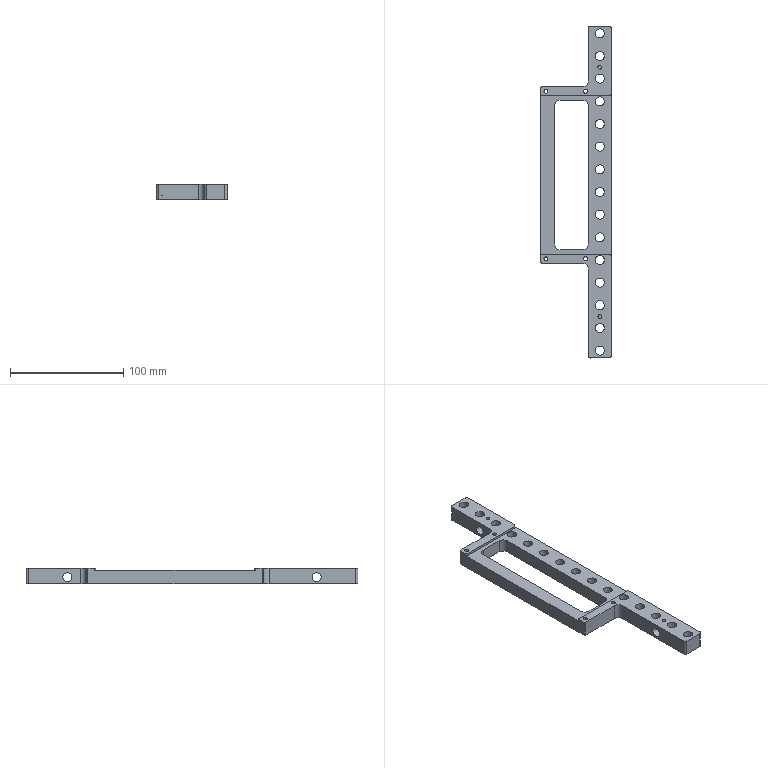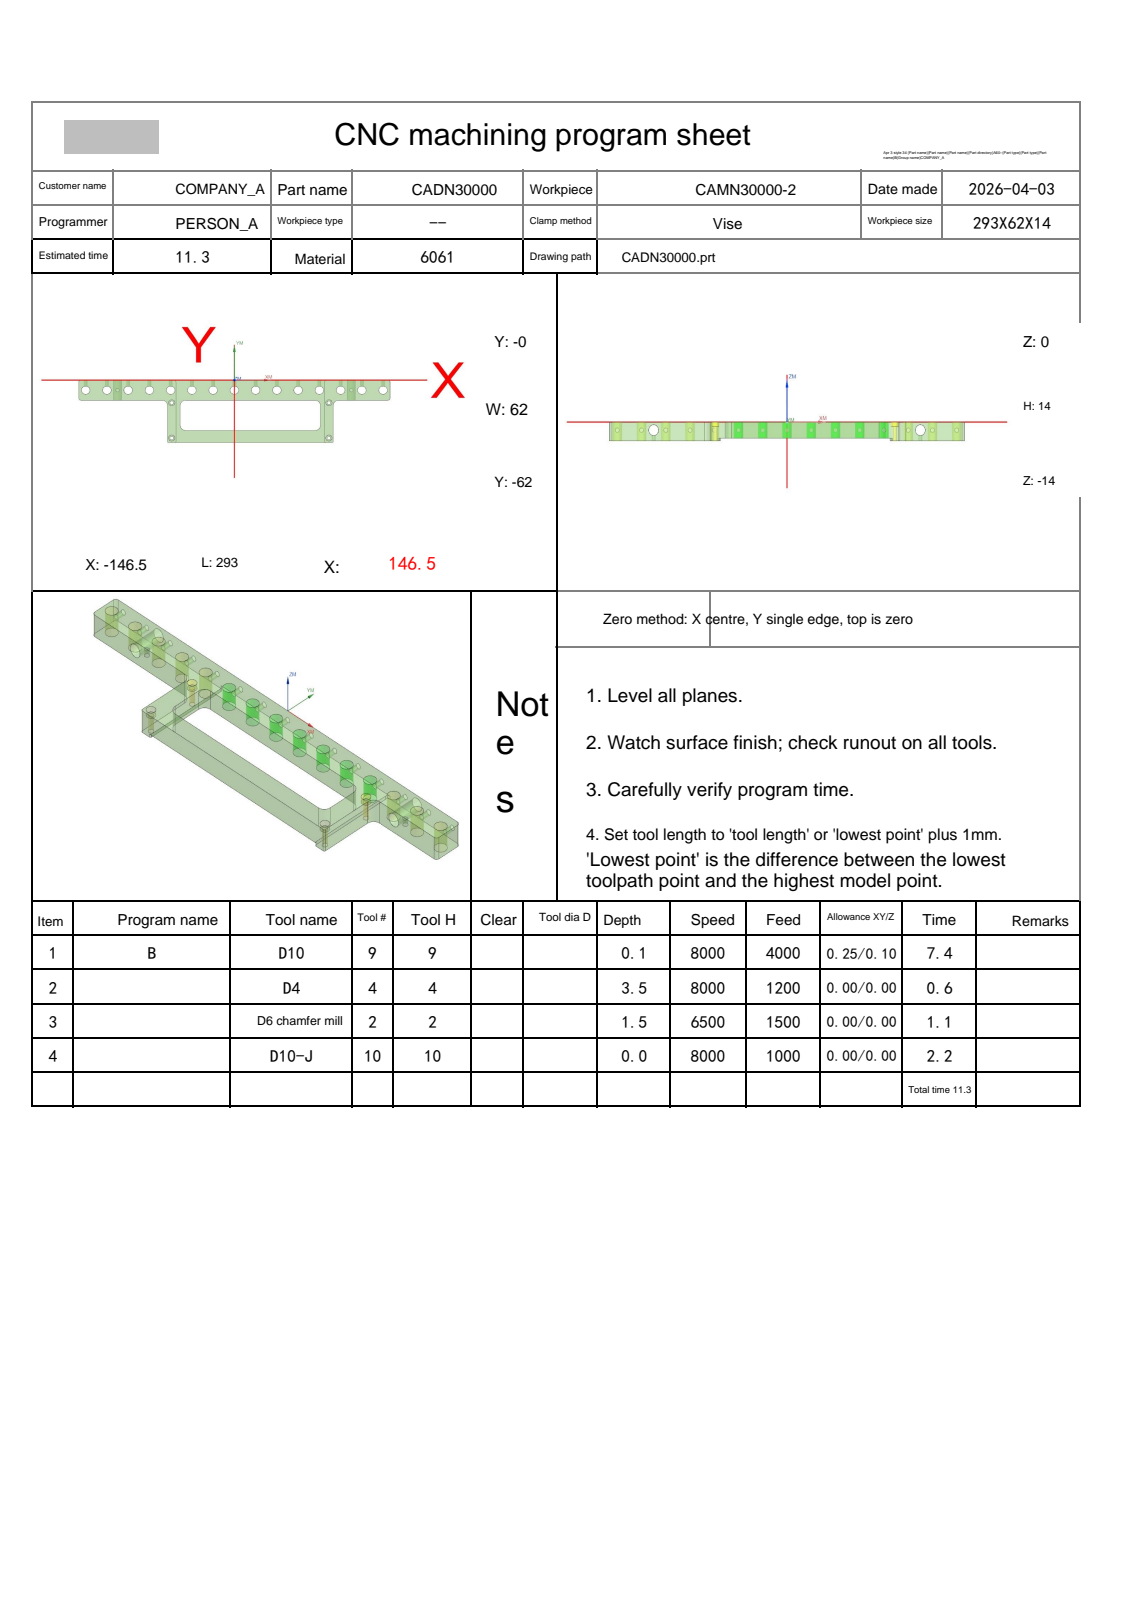NC program | NX | posted by the shop | part box 62 x 293 x 14 mm
Lines 1 to 1541 of 1949, first 1264 of 1539 lines:
%
O0001
(Machine time: 11.99 MIN)
(===Total Tool:4===)
(T9=D10     D=10.  R=0.   D-  H09 Z=0.1   )
(T4=D4      D=4.   R=0.   D-  H04 Z=-3.5  )
(T2=D6 chamfer mill   D=6.   R=0.   D-  H02 Z=-1.5  )
(T10=D10-J  D=10.  R=0.   D-  H10 Z=-0.   )
G80 G90 G17 G49 G40
G91 G28 Z0
M01
N1 T09 M06
(D10  D=10. R=0. H=09 ce=0.25 di=0.10)
G00 G90 G54 X88.84 Y12.6 M03 S8000
G43 H09 Z20.
M08
Z2.1
G01 X88.857 Y12.502 Z1.476 F4000.
X88.874 Y12.403 Z1.228
X88.891 Y12.305 Z1.046
X88.908 Y12.206 Z.9
X88.925 Y12.108 Z.777
X88.943 Y12.009 Z.672
X88.96 Y11.911 Z.58
X88.977 Y11.812 Z.5
X88.994 Y11.714 Z.43
X89.011 Y11.615 Z.368
X89.028 Y11.516 Z.314
X89.045 Y11.418 Z.267
X89.062 Y11.319 Z.227
X89.079 Y11.221 Z.192
X89.096 Y11.122 Z.164
X89.113 Y11.024 Z.14
X89.13 Y10.925 Z.123
X89.147 Y10.827 Z.11
X89.164 Y10.728 Z.103
X89.181 Y10.63 Z.1
X89.568 Y8.389
G03 X89.885 Y8.003 I.502 J.09
X93.672 Y7.43 I3.807 J12.364
X102.367 Y7.294 I8.695 J277.549
X104.221 Y7.3 I0.0 J277.686
G01 X147.34 Y7.279
G02 X153.274 Y3.249 I-.2 J-6.678
X154.598 Y-2.599 I-14.948 J-6.46
X154.816 Y-11.507 I-182.121 J-8.909
X154.799 Y-14.005 I-182.338 J0.0
G01 X154.782 Y-61.787
G02 X150.627 Y-67.842 I-6.717 J.156
X144.706 Y-69.114 I-6.461 J15.657
X136.65 Y-69.305 I-8.056 J169.876
X135.049 Y-69.297 I0.0 J170.067
G01 X-147.307 Y-69.281
G02 X-153.303 Y-65.187 I.18 J6.701
X-154.592 Y-59.479 I14.994 J6.386
X-154.808 Y-51.337 I153.279 J8.142
X-154.798 Y-49.543 I153.495 J0.0
G01 X-154.781 Y-.193
G02 X-150.823 Y5.737 I6.655 J-.155
X-145.06 Y7.085 I6.436 J-14.522
X-136.504 Y7.313 I8.556 J-160.42
X-134.285 Y7.298 I0.0 J-160.648
G01 X87.395 Y7.279
G03 X96.14 Y6.68 I14.491 J147.608
X105.341 Y6.601 I9.81 J603.736
G01 X145.58 Y6.575
G02 X152.002 Y2.432 I-.439 J-7.729
X153.748 Y-3.652 I-14.055 J-7.328
X154.101 Y-11.947 I-97.334 J-8.296
X154.092 Y-13.301 I-97.687 J0.0
G01 X154.082 Y-59.92
G02 X149.837 Y-66.561 I-7.749 J.276
X143.738 Y-68.262 I-7.302 J14.397
X135.453 Y-68.601 I-8.285 J101.008
X134.088 Y-68.592 I0.0 J101.348
G01 X-145.58 Y-68.575
G02 X-152.029 Y-64.382 I.448 J7.745
X-153.755 Y-58.288 I14.212 J7.317
X-154.11 Y-49.527 I108.129 J8.761
X-154.095 Y-47.728 I108.483 J0.0
G01 X-154.075 Y-1.921
G02 X-149.934 Y4.499 I7.732 J-.442
X-143.711 Y6.263 I7.389 J-14.205
X-135.007 Y6.609 I8.704 J-109.461
X-133.221 Y6.594 I0.0 J-109.807
G01 X85.659 Y6.584
G02 X94.023 Y6.08 I-43.845 J-798.073
G03 X105.145 Y5.898 I11.123 J339.757
X106.531 Y5.901 I0.0 J339.939
G01 X143.761 Y5.877
G02 X151.325 Y.864 I-.379 J-8.787
X153.058 Y-5.735 I-16.655 J-7.9
X153.409 Y-15.038 I-123.06 J-9.303
X153.395 Y-16.926 I-123.411 J0.0
G01 X153.375 Y-58.285
G02 X148.444 Y-65.787 I-8.757 J.384
X141.717 Y-67.564 I-7.966 J16.537
X132.386 Y-67.909 I-9.331 J125.76
X130.456 Y-67.895 I0.0 J126.105
G01 X-143.723 Y-67.877
G02 X-151.337 Y-62.841 I.347 J8.797
X-153.067 Y-56.172 I16.812 J7.921
X-153.409 Y-46.885 I126.17 J9.288
X-153.395 Y-44.981 I126.512 J0.0
G01 X-153.377 Y-3.761
G02 X-148.442 Y3.784 I8.769 J-.349
X-141.847 Y5.549 I7.91 J-16.351
X-133.209 Y5.897 I8.638 J-107.04
X-131.987 Y5.89 I0.0 J-107.388
G01 X84.723 Y5.876
G02 X94.905 Y5.361 I-44.85 J-988.753
G03 X107.105 Y5.198 I12.2 J456.693
X108.841 Y5.202 I0.0 J456.856
G01 X142.01 Y5.179
G02 X150.616 Y-.477 I-.151 J-9.604
X152.35 Y-7.374 I-18.435 J-8.3
X152.71 Y-17.163 I-132.671 J-9.789
X152.695 Y-19.195 I-133.032 J0.0
G01 X152.678 Y-56.495
G02 X147.046 Y-65.107 I-9.589 J.123
X140.091 Y-66.854 I-8.325 J18.431
X130.3 Y-67.21 I-9.791 J134.473
X128.27 Y-67.194 I0.0 J134.829
G01 X-141.99 Y-67.177
G02 X-150.618 Y-61.517 I.129 J9.603
X-152.37 Y-54.413 I18.732 J8.387
X-152.702 Y-45.095 I130.593 J9.318
X-152.693 Y-43.501 I130.925 J0.0
G01 X-152.677 Y-5.501
G02 X-147.023 Y3.116 I9.604 J-.138
X-140.126 Y4.849 I8.3 J-18.445
X-130.723 Y5.203 I9.403 J-124.716
X-129.075 Y5.192 I0.0 J-125.07
G01 X83.715 Y5.175
G02 X94.918 Y4.674 I-31.295 J-824.645
G03 X108.198 Y4.496 I13.28 J497.487
X110.451 Y4.502 I0.0 J497.664
G01 X140.4 Y4.479
X140.468 Y4.48
G02 X149.953 Y-1.808 I0.0 J-10.298
X151.663 Y-9.069 I-20.482 J-8.658
X152.004 Y-18.858 I-140.517 J-9.788
X151.993 Y-20.611 I-140.858 J0.0
G01 X151.98 Y-54.831
X151.981 Y-54.97
G02 X148.938 Y-62.275 I-10.291 J0.0
X142.504 Y-65.531 I-9.145 J10.086
X133.954 Y-66.411 I-8.704 J42.604
X122.796 Y-66.502 I-11.158 J686.931
X120.655 Y-66.498 I0.0 J687.022
G01 X-140.295 Y-66.481
X-140.451 Y-66.482
G02 X-147.553 Y-63.657 I0.0 J10.341
X-151.023 Y-57.031 I9.674 J9.288
X-151.912 Y-48.412 I42.61 J8.75
X-152.002 Y-37.319 I686.42 J11.093
X-151.998 Y-35.183 I686.51 J0.0
G01 X-151.975 Y-7.053
Y-7.023
G02 X-145.736 Y2.433 I10.284 J0.0
X-138.343 Y4.171 I8.722 J-20.502
X-128.525 Y4.504 I9.818 J-144.463
X-126.731 Y4.493 I0.0 J-144.796
G01 X82.559 Y4.479
G02 X95.738 Y3.957 I-29.69 J-915.635
G03 X109.111 Y3.801 I13.373 J573.724
X110.241 Y3.802 I0.0 J573.88
G01 X138.93 Y3.779
X139.056
G02 X145.641 Y1.684 I0.0 J-11.398
X149.894 Y-4.682 I-7.718 J-9.76
X151.13 Y-12.967 I-31.784 J-8.976
X151.314 Y-24.728 I-376.482 J-11.761
X151.298 Y-28.155 I-376.666 J0.0
G01 X151.279 Y-53.345
X151.28 Y-53.52
G02 X149.36 Y-59.899 I-11.556 J0.0
X142.994 Y-64.339 I-9.814 J7.288
X134.787 Y-65.617 I-8.967 J30.583
X122.844 Y-65.816 I-11.944 J359.429
X119.25 Y-65.798 I0.0 J359.627
G01 X-138.83 Y-65.779
X-139.013 Y-65.78
G02 X-145.447 Y-63.823 I0.0 J11.554
X-149.891 Y-57.325 I7.423 J9.846
X-151.13 Y-49.04 I31.759 J8.982
X-151.314 Y-37.2 I380.01 J11.84
X-151.298 Y-33.712 I380.194 J0.0
G01 X-151.277 Y-8.592
X-151.278 Y-8.446
G02 X-149.201 Y-1.884 I11.406 J0.0
X-142.754 Y2.414 I9.788 J-7.698
X-134.745 Y3.619 I8.836 J-31.512
X-122.8 Y3.816 I11.946 J-362.968
X-119.208 Y3.798 I0.0 J-363.165
G01 X81.682 Y3.78
G02 X95.597 Y3.269 I-21.781 J-783.97
G03 X110.152 Y3.097 I14.555 J615.329
X112.55 Y3.102 I0.0 J615.501
G01 X137.53 Y3.079
X137.685
G02 X143.897 Y1.449 I0.0 J-12.646
X148.895 Y-4.964 I-6.518 J-10.234
X150.361 Y-13.135 I-27.913 J-9.224
X150.606 Y-23.713 I-228.264 J-10.577
X150.596 Y-25.871 I-228.509 J0.0
G01 X150.577 Y-51.971
X150.579 Y-52.167
G02 X148.98 Y-58.347 I-12.741 J0.0
X142.64 Y-63.357 I-10.219 J6.415
X134.474 Y-64.854 I-9.244 J27.407
X123.793 Y-65.107 I-10.681 J225.167
X121.528 Y-65.095 I0.0 J225.42
G01 X-137.462 Y-65.077
G02 X-137.662 Y-65.078 I-.2 J12.731
X-143.906 Y-63.442 I0.0 J12.733
X-148.872 Y-57.094 I6.52 J10.217
X-150.352 Y-48.996 I27.485 J9.206
X-150.607 Y-38.319 I223.444 J10.677
X-150.595 Y-36.05 I223.699 J0.0
G01 X-150.572 Y-9.88
X-150.573 Y-9.75
G02 X-148.751 Y-3.29 I12.364 J0.0
X-142.272 Y1.488 I10.176 J-7.017
X-134.29 Y2.865 I9.093 J-28.888
X-123.711 Y3.105 I10.579 J-233.001
X-121.554 Y3.095 I0.0 J-233.241
G01 X81.506 Y3.072
G02 X96.008 Y2.564 I-25.441 J-933.963
G03 X110.8 Y2.4 I14.791 J665.06
X112.621 Y2.402 I0.0 J665.225
G01 X136.13 Y2.38
G02 X136.35 Y2.382 I.22 J-13.999
X142.43 Y.993 I0.0 J-14.001
X148.029 Y-5.615 I-5.888 J-10.665
X149.614 Y-13.762 I-26.727 J-9.429
X149.914 Y-25.328 I-223.098 J-11.567
X149.896 Y-28.176 I-223.398 J0.0
G01 X149.87 Y-50.846
X149.871 Y-50.979
G02 X148.288 Y-57.303 I-13.428 J0.0
X141.67 Y-62.611 I-10.58 J6.412
X133.648 Y-64.121 I-9.33 J27.506
X122.041 Y-64.414 I-11.607 J230.015
X119.163 Y-64.396 I0.0 J230.308
G01 X-136.117 Y-64.376
G02 X-136.342 Y-64.378 I-.226 J14.074
X-142.355 Y-63.029 I0.0 J14.076
X-147.964 Y-56.545 I5.746 J10.639
X-149.606 Y-48.341 I26.119 J9.494
X-149.902 Y-37.833 I186.436 J10.507
X-149.893 Y-35.956 I186.732 J0.0
G01 X-149.875 Y-11.327
G02 X-149.876 Y-11.119 I13.86 J.208
X-148.438 Y-4.97 I13.861 J0.0
X-141.87 Y.533 I10.622 J-6.005
X-133.931 Y2.099 I9.336 J-26.426
X-122.586 Y2.412 I11.345 J-205.627
X-119.937 Y2.395 I0.0 J-205.939
G01 X80.743 Y2.373
G02 X96.006 Y1.87 I-21.929 J-897.113
G03 X111.368 Y1.7 I15.363 J692.97
X113.251 Y1.703 I0.0 J693.14
G01 X134.94 Y1.677
G02 X135.156 Y1.679 I.215 J-14.903
X141.327 Y.341 I0.0 J-14.904
X147.13 Y-6.162 I-5.666 J-10.896
X148.853 Y-14.207 I-25.216 J-9.608
X149.194 Y-24.497 I-154.696 J-10.291
X149.188 Y-25.889 I-155.038 J0.0
G01 X149.176 Y-49.328
G02 X149.178 Y-49.599 I-15.233 J-.271
X147.919 Y-55.664 I-15.236 J0.0
X141.254 Y-61.665 I-10.984 J5.499
X133.342 Y-63.348 I-9.53 J25.353
X122.945 Y-63.696 I-10.396 J155.45
X121.45 Y-63.688 I0.0 J155.798
G01 X-134.74 Y-63.678
G02 X-135.041 Y-63.681 I-.301 J15.542
X-141.024 Y-62.483 I0.0 J15.545
X-147.102 Y-55.9 I5.294 J10.986
X-148.846 Y-47.859 I24.933 J9.619
X-149.197 Y-37.382 I156.383 J10.477
X-149.189 Y-35.827 I156.734 J0.0
G01 X-149.174 Y-12.597
G02 X-149.176 Y-12.375 I15.13 J.223
X-147.916 Y-6.33 I15.132 J0.0
X-141.331 Y-.369 I10.951 J-5.479
X-133.076 Y1.37 I9.701 J-25.588
X-121.622 Y1.71 I11.454 J-192.661
X-119.083 Y1.694 I0.0 J-193.001
G01 X79.847 Y1.676
G02 X95.726 Y1.183 I-17.854 J-830.973
G03 X111.743 Y1. I16.017 J699.437
X113.811 Y1.003 I0.0 J699.62
G01 X133.751 Y.976
G02 X133.967 Y.978 I.217 J-15.98
X140.163 Y-.272 I0.0 J-15.981
X146.322 Y-6.909 I-5.414 J-11.201
X148.114 Y-14.939 I-24.864 J-9.764
X148.498 Y-25.765 I-152.549 J-10.826
X148.489 Y-27.459 I-152.932 J0.0
G01 X148.477 Y-48.029
G02 X148.48 Y-48.32 I-16.947 J-.291
X147.426 Y-54.203 I-16.95 J0.0
X140.619 Y-60.81 I-11.344 J4.878
X132.453 Y-62.624 I-9.826 J24.94
X121.138 Y-63.005 I-11.314 J167.762
X118.952 Y-62.991 I0.0 J168.143
G01 X-133.528 Y-62.977
G02 X-133.84 Y-62.98 I-.311 J16.739
X-139.832 Y-61.871 I0.0 J16.742
X-146.328 Y-55.072 I5.033 J11.312
X-148.14 Y-46.762 I25.364 J9.884
X-148.493 Y-36.299 I154.908 J10.464
X-148.488 Y-34.941 I155.261 J0.0
G01 X-148.469 Y-13.671
X-148.47 Y-13.481
G02 X-147.192 Y-7.263 I15.756 J0.0
X-140.432 Y-1.113 I11.22 J-5.541
X-132.25 Y.642 I9.799 J-25.742
X-121.093 Y1.003 I11.157 J-171.958
X-119.028 Y.991 I0.0 J-172.32
G01 X79.762 Y.971
G02 X96.624 Y.464 I-21.139 J-983.732
G03 X112.277 Y.3 I15.653 J748.037
X114.581 Y.303 I0.0 J748.201
G01 X132.421 Y.28
G02 X132.72 Y.283 I.299 J-17.568
X138.868 Y-.828 I0.0 J-17.571
X145.525 Y-7.656 I-4.993 J-11.526
X147.398 Y-15.88 I-24.884 J-9.993
X147.795 Y-26.763 I-148.941 J-10.883
X147.787 Y-28.33 I-149.338 J0.0
G01 X147.776 Y-46.87
G02 X147.779 Y-47.187 I-17.896 J-.317
X146.742 Y-53.19 I-17.898 J0.0
X139.839 Y-60.026 I-11.586 J4.795
X131.749 Y-61.886 I-9.936 J24.704
X120.994 Y-62.292 I-10.755 J142.146
X119.579 Y-62.285 I0.0 J142.553
G01 X-132.411 Y-62.275
G02 X-132.712 Y-62.277 I-.302 J17.679
X-138.793 Y-61.199 I0.0 J17.682
X-145.577 Y-54.22 I4.939 J11.588
X-147.423 Y-45.841 I25.625 J10.039
X-147.802 Y-34.57 I167.216 J11.271
X-147.79 Y-32.55 I167.595 J0.0
X-147.818 Y-25.468 I917.727 J7.082
X-147.749 Y-14.29 I917.754 J0.0
X-146.216 Y-7.665 I15.196 J-.027
X-139.246 Y-1.729 I11.361 J-6.281
X-130.692 Y-.023 I10.03 J-27.99
X-119.024 Y.307 I11.668 J-205.842
X-116.559 Y.293 I0.0 J-206.173
G01 X78.801 Y.275
G02 X96.138 Y-.22 I-16.782 J-892.922
G03 X112.269 Y-.397 I16.131 J732.322
X113.671 Y-.396 I0.0 J732.5
G02 X120.248 Y-.373 I6.577 J-953.697
X132.14 Y-.447 I0.0 J-953.72
X138.848 Y-1.95 I-.036 J-15.888
X144.958 Y-8.922 I-6.153 J-11.555
X146.724 Y-17.245 I-26.973 J-10.07
X147.102 Y-28.693 I-172.99 J-11.448
X147.09 Y-30.746 I-173.368 J0.0
X147.115 Y-36.628 I-678.98 J-5.881
X147.039 Y-46.836 I-679.006 J0.0
X145.425 Y-53.584 I-15.389 J.113
X138.313 Y-59.562 I-11.546 J6.516
X129.971 Y-61.247 I-10.024 J28.129
X118.505 Y-61.602 I-11.466 J185.038
X116.399 Y-61.59 I0.0 J185.393
G01 X-131.041 Y-61.579
G02 X-131.448 Y-61.583 I-.406 J19.659
X-137.519 Y-60.622 I0.0 J19.664
X-144.667 Y-53.748 I4.483 J11.815
X-146.656 Y-45.472 I24.145 J10.179
X-147.092 Y-34.477 I138.445 J10.995
X-147.084 Y-33.024 I138.881 J0.0
X-147.119 Y-25.987 I713.915 J7.037
X-147.036 Y-15.115 I713.95 J0.0
X-145.332 Y-8.25 I15.214 J-.132
X-138.254 Y-2.416 I11.493 J-6.734
X-129.699 Y-.731 I10.113 J-28.783
X-117.962 Y-.394 I11.737 J-204.191
X-115.566 Y-.408 I0.0 J-204.528
G01 X78.744 Y-.43
G02 X96.691 Y-.93 I-18.209 J-976.343
G03 X112.38 Y-1.097 I15.688 J736.431
X113.952 Y-1.096 I0.0 J736.598
G02 X119.766 Y-1.076 I5.815 J-886.428
X131.09 Y-1.149 I0.0 J-886.447
X137.879 Y-2.621 I-.036 J-16.56
X144.238 Y-9.806 I-6.085 J-11.791
X146.033 Y-18.415 I-27.816 J-10.293
X146.399 Y-29.803 I-177.212 J-11.388
X146.389 Y-31.707 I-177.578 J0.0
X146.416 Y-36.797 I-477.543 J-5.09
X146.328 Y-45.976 I-477.571 J0.0
X144.631 Y-52.851 I-15.592 J.2
X137.496 Y-58.815 I-11.676 J6.718
X128.881 Y-60.55 I-10.255 J28.671
X117.36 Y-60.901 I-11.521 J188.871
X115.308 Y-60.889 I0.0 J189.222
G01 X-130.102 Y-60.874
G02 X-130.451 Y-60.877 I-.349 J20.105
X-136.649 Y-59.898 I0.0 J20.108
X-144.034 Y-52.674 I4.584 J12.072
X-145.986 Y-44.108 I25.711 J10.367
X-146.393 Y-32.944 I152.908 J11.164
X-146.385 Y-31.378 I153.315 J0.0
X-146.411 Y-25.725 I615.598 J5.653
X-146.339 Y-16.269 I615.624 J0.0
X-144.811 Y-9.493 I16.199 J-.092
X-137.657 Y-3.249 I11.767 J-6.263
X-129.331 Y-1.489 I10.156 J-27.461
X-117.553 Y-1.097 I11.778 J-176.771
X-115.341 Y-1.111 I0.0 J-177.163
G01 X77.919 Y-1.127
G02 X96.898 Y-1.632 I-16.767 J-987.844
G03 X113.01 Y-1.8 I16.113 J772.234
X115.631 Y-1.796 I0.0 J772.402
G02 X120.526 Y-1.772 I4.895 J-515.491
X130.46 Y-1.868 I0.0 J-515.514
X137.352 Y-3.506 I-.209 J-16.2
X143.498 Y-10.622 I-6.524 J-11.846
X145.302 Y-19.08 I-27.657 J-10.321
X145.699 Y-30.739 I-170.736 J-11.659
X145.688 Y-32.721 I-171.133 J0.0
X145.713 Y-36.965 I-355.109 J-4.244
X145.622 Y-45.04 I-355.134 J0.0
X143.852 Y-52.107 I-15.867 J.217
X136.666 Y-58.081 I-11.807 J6.893
X127.844 Y-59.85 I-10.457 J29.261
X116.373 Y-60.198 I-11.472 J189.114
X114.482 Y-60.188 I0.0 J189.462
G01 X-128.828 Y-60.177
G02 X-129.263 Y-60.182 I-.435 J21.991
X-135.462 Y-59.29 I0.0 J21.995
X-143.192 Y-52.081 I4.23 J12.285
X-145.206 Y-43.891 I24.404 J10.342
X-145.682 Y-32.885 I126.938 J11.006
X-145.678 Y-31.795 I127.415 J0.0
X-145.712 Y-26.055 I477.085 J5.74
X-145.628 Y-17.096 I477.12 J0.0
X-143.983 Y-10.138 I16.25 J-.169
X-136.989 Y-4.05 I11.801 J-6.495
X-128.607 Y-2.216 I10.309 J-27.045
X-116.774 Y-1.799 I11.832 J-167.737
X-114.687 Y-1.812 I0.0 J-168.154
G01 X77.243 Y-1.826
G02 X95.786 Y-2.301 I-12.828 J-862.502
G03 X113.332 Y-2.499 I17.546 J779.587
X115.771 Y-2.495 I0.0 J779.784
G02 X120.317 Y-2.471 I4.546 J-432.564
X129.41 Y-2.567 I0.0 J-432.588
X136.259 Y-4.097 I-.192 J-16.957
X142.718 Y-11.325 I-6.241 J-12.076
X144.586 Y-19.912 I-27.533 J-10.488
X144.992 Y-31.295 I-159.616 J-11.383
X144.984 Y-32.852 I-160.021 J0.0
X145.012 Y-36.73 I-266.211 J-3.878
X144.904 Y-44.331 I-266.239 J0.0
X143. Y-51.503 I-15.76 J.344
X135.896 Y-57.329 I-11.849 J7.204
X127.426 Y-59.1 I-10.382 J28.51
X115.611 Y-59.499 I-11.815 J174.826
X113.576 Y-59.487 I0.0 J175.225
G01 X-127.774 Y-59.477
G02 X-128.22 Y-59.481 I-.446 J23.007
X-134.484 Y-58.612 I0.0 J23.011
X-142.48 Y-51.218 I4.142 J12.5
X-144.515 Y-42.818 I25.05 J10.514
X-144.981 Y-31.75 I131.043 J11.068
X-144.977 Y-30.722 I131.51 J0.0
X-145.01 Y-25.939 I346.229 J4.782
X-144.917 Y-17.913 I346.262 J0.0
X-143.254 Y-10.958 I16.445 J-.257
X-136.048 Y-4.733 I11.992 J-6.599
X-127.241 Y-2.884 I10.568 J-28.442
X-115.538 Y-2.502 I11.702 J-179.234
X-113.599 Y-2.513 I0.0 J-179.616
G01 X77.21 Y-2.53
G02 X95.854 Y-3.001 I-12.846 J-878.812
G03 X116.428 Y-3.218 I20.574 J974.307
X123.041 Y-3.195 I0.0 J974.524
G02 X124.647 Y-3.176 I1.606 J-65.16
X130.661 Y-3.454 I0.0 J-65.179
X141.844 Y-11.796 I-1.292 J-13.397
X143.842 Y-20.424 I-26.388 J-10.658
X144.293 Y-32.187 I-153.104 J-11.763
X144.284 Y-33.922 I-153.556 J0.0
X144.314 Y-37.028 I-161.417 J-3.106
X144.169 Y-43.859 I-161.446 J0.0
X141.909 Y-51.282 I-15.196 J.572
X134.502 Y-56.82 I-11.909 J8.207
X125.511 Y-58.475 I-10.594 J32.302
X112.98 Y-58.807 I-12.531 J236.215
X110.257 Y-58.791 I0.0 J236.547
G01 X-126.753 Y-58.776
G02 X-127.199 Y-58.78 I-.446 J24.022
X-133.536 Y-57.929 I0.0 J24.026
X-141.768 Y-50.367 I4.075 J12.698
X-143.831 Y-41.688 I25.767 J10.708
X-144.294 Y-29.883 I150.222 J11.805
X-144.283 Y-28.12 I150.685 J0.0
X-144.315 Y-24.971 I155.561 J3.149
X-144.161 Y-18.043 I155.593 J0.0
X-141.892 Y-10.695 I15.057 J-.625
X-134.728 Y-5.265 I11.822 J-8.156
X-126.1 Y-3.571 I10.467 J-30.498
X-114.431 Y-3.204 I11.67 J-185.468
X-112.598 Y-3.213 I0.0 J-185.835
G01 X76.531 Y-3.229
G02 X96.131 Y-3.705 I-12.158 J-903.17
G03 X116.738 Y-3.919 I20.607 J993.612
X123.391 Y-3.897 I0.0 J993.826
G02 X124.616 Y-3.88 I1.226 J-44.242
X130.72 Y-4.303 I0.0 J-44.259
X141.022 Y-12.389 I-2.133 J-13.323
X143.118 Y-21.132 I-25.91 J-10.833
X143.587 Y-32.765 I-143.885 J-11.633
X143.58 Y-34.209 I-144.354 J0.0
X143.609 Y-36.858 I-121.762 J-2.649
X143.442 Y-43.236 I-121.791 J0.0
X140.97 Y-50.795 I-15.02 J.726
X133.738 Y-56.078 I-11.864 J8.651
X124.679 Y-57.764 I-10.706 J32.336
X111.98 Y-58.107 I-12.699 J235.208
X109.215 Y-58.091 I0.0 J235.55
G01 X-125.695 Y-58.076
G02 X-126.153 Y-58.08 I-.458 J25.45
X-132.487 Y-57.279 I0.0 J25.454
X-141.022 Y-49.604 I3.881 J12.899
X-143.103 Y-41.001 I25.677 J10.765
X-143.581 Y-29.634 I134.949 J11.367
X-143.576 Y-28.484 I135.427 J0.0
X-143.608 Y-25.489 I139.269 J2.995
X-143.452 Y-18.897 I139.301 J0.0
X-141.125 Y-11.431 I15.277 J-.666
X-133.816 Y-5.952 I11.962 J-8.341
X-124.696 Y-4.237 I10.751 J-32.075
X-111.947 Y-3.893 I12.749 J-235.651
X-109.162 Y-3.909 I0.0 J-235.996
G01 X75.908 Y-3.928
G02 X96.616 Y-4.415 I-11.981 J-949.517
G03 X116.691 Y-4.618 I20.075 J990.377
X122.971 Y-4.598 I0.0 J990.581
G02 X123.981 Y-4.586 I1.011 J-40.299
X130.086 Y-5.051 I0.0 J-40.312
X140.262 Y-13.111 I-2.343 J-13.411
X142.357 Y-21.502 I-25.228 J-10.756
X142.883 Y-33.257 I-131.152 J-11.755
X142.876 Y-34.576 I-131.677 J0.0
X142.908 Y-36.821 I-80.131 J-2.244
X142.661 Y-43.109 I-80.162 J0.0
X139.12 Y-51.405 I-14.081 J1.107
X131.646 Y-55.778 I-11.638 J11.317
X122.318 Y-57.154 I-10.684 J40.112
X108.766 Y-57.412 I-13.551 J356.426
X105.101 Y-57.393 I0.0 J356.683
G01 X-124.979 Y-57.37
G02 X-125.354 Y-57.373 I-.375 J24.826
X-131.832 Y-56.513 I0.0 J24.829
X-140.281 Y-48.842 I4.065 J12.965
X-142.377 Y-40.313 I25.583 J10.81
X-142.883 Y-28.628 I134.625 J11.686
X-142.877 Y-27.308 I135.132 J0.0
X-142.907 Y-25.122 I79.321 J2.186
X-142.664 Y-18.916 I79.351 J0.0
X-139.217 Y-10.704 I14.123 J-1.099
X-131.564 Y-6.199 I11.734 J-11.18
X-122.093 Y-4.834 I10.73 J-40.9
X-108.583 Y-4.589 I13.51 J-373.067
X-104.946 Y-4.607 I0.0 J-373.311
G01 X76.064 Y-4.633
G02 X96.615 Y-5.113 I-12.151 J-960.456
G03 X116.755 Y-5.318 I20.14 J988.296
X122.481 Y-5.301 I0.0 J988.501
G02 X123.323 Y-5.292 I.842 J-37.064
X129.521 Y-5.813 I0.0 J-37.074
X139.548 Y-13.924 I-2.615 J-13.486
X141.661 Y-22.456 I-25.653 J-10.879
X142.182 Y-34.266 I-133.461 J-11.81
X142.175 Y-35.67 I-133.983 J0.0
X142.199 Y-37.187 I-47.579 J-1.517
X141.789 Y-43.421 I-47.603 J0.0
X133.442 Y-54.107 I-13.627 J2.042
X124.554 Y-56.212 I-11.01 J26.675
X112.585 Y-56.688 I-11.969 J149.964
X110.987 Y-56.68 I0.0 J150.441
G01 X-123.713 Y-56.675
G02 X-124.178 Y-56.679 I-.465 J27.614
X-130.583 Y-55.926 I0.0 J27.618
X-139.466 Y-48.245 I3.625 J13.17
X-141.662 Y-39.526 I25.241 J10.992
X-142.184 Y-27.633 I135.276 J11.893
X-142.175 Y-26.101 I135.798 J0.0
X-142.197 Y-24.694 I45.961 J1.407
X-141.786 Y-18.561 I45.982 J0.0
X-133.515 Y-7.928 I13.62 J-2.061
X-124.846 Y-5.819 I10.929 J-26.053
X-113.284 Y-5.322 I11.562 J-134.198
X-112.191 Y-5.326 I0.0 J-134.695
G01 X75.469 Y-5.331
G02 X95.502 Y-5.784 I-9.603 J-868.534
G03 X116.571 Y-6.015 I21.07 J958.587
X121.643 Y-6.002 I0.0 J958.818
G02 X122.5 Y-5.992 I.858 J-35.875
X128.956 Y-6.577 I0.0 J-35.885
X138.829 Y-14.716 I-2.881 J-13.552
X140.97 Y-23.45 I-26.109 J-11.031
X141.469 Y-34.672 I-126.028 J-11.222
X141.34 Y-40.372 I-126.527 J0.0
X139.19 Y-47.837 I-16.265 J.643
X131.728 Y-53.771 I-12.386 J7.917
X122.632 Y-55.604 I-10.98 J30.996
X110.584 Y-55.993 I-12.049 J186.572
X108.781 Y-55.984 I0.0 J186.961
G01 X-122.699 Y-55.975
G02 X-123.205 Y-55.979 I-.506 J28.622
X-129.711 Y-55.23 I0.0 J28.627
X-138.767 Y-47.414 I3.596 J13.32
X-140.946 Y-38.759 I25.489 J11.022
X-141.471 Y-27.398 I122.686 J11.361
X-141.33 Y-21.489 I123.211 J0.0
X-139.081 Y-13.99 I16.013 J-.715
X-131.487 Y-8.14 I12.387 J-8.226
X-122.306 Y-6.37 I10.98 J-32.264
X-110.463 Y-6.009 I11.843 J-194.176
X-108.804 Y-6.016 I0.0 J-194.537
G01 X74.866 Y-6.03
G02 X96.892 Y-6.515 I-10.818 J-992.529
G03 X116.883 Y-6.716 I19.992 J991.098
X121.224 Y-6.707 I0.0 J991.3
G02 X121.918 Y-6.699 I.695 J-32.672
X128.527 Y-7.375 I0.0 J-32.679
X138.122 Y-15.529 I-3.285 J-13.589
X140.276 Y-24.405 I-26.524 J-11.136
X140.752 Y-34.287 I-102.535 J-9.882
X140.597 Y-39.927 I-103.011 J0.0
X138.057 Y-47.692 I-15.656 J.823
X130.466 Y-53.229 I-12.323 J8.923
X121.479 Y-54.924 I-10.913 J33.197
X109.303 Y-55.293 I-12.175 J200.42
X107.416 Y-55.285 I0.0 J200.79
G01 X-121.824 Y-55.273
G02 X-122.332 Y-55.278 I-.508 J28.747
X-128.972 Y-54.501 I0.0 J28.751
X-138.078 Y-46.563 I3.7 J13.436
X-140.25 Y-37.837 I25.968 J11.097
X-140.748 Y-27.602 I104.879 J10.235
X-140.612 Y-22.246 I105.377 J0.0
X-138.31 Y-14.691 I16.02 J-.752
X-130.876 Y-8.924 I12.392 J-8.3
X-121.776 Y-7.1 I11.032 J-31.431
X-109.612 Y-6.708 I12.164 J-188.165
X-107.784 Y-6.716 I0.0 J-188.558
G01 X74.276 Y-6.729
G02 X95.917 Y-7.19 I-8.438 J-903.489
G03 X116.692 Y-7.415 I20.775 J962.852
X120.385 Y-7.407 I0.0 J963.076
G02 X121.027 Y-7.401 I.642 J-33.371
X127.621 Y-8.059 I0.0 J-33.377
X137.319 Y-16.123 I-3.167 J-13.674
X139.543 Y-24.977 I-25.944 J-11.221
X140.02 Y-34.194 I-88.825 J-9.217
X139.889 Y-39.028 I-89.302 J0.0
X137.413 Y-46.812 I-15.926 J.779
X129.718 Y-52.499 I-12.465 J8.817
X120.526 Y-54.228 I-11.06 J33.507
X108.521 Y-54.589 I-12.005 J199.196
X106.883 Y-54.583 I0.0 J199.557
G01 X-120.886 Y-54.573
G02 X-121.407 Y-54.578 I-.52 J29.567
X-128.108 Y-53.808 I0.0 J29.572
X-137.352 Y-45.802 I3.644 J13.547
X-139.537 Y-37.072 I26.019 J11.151
X-140.023 Y-27.912 I86.134 J9.16
X-139.868 Y-22.742 I86.62 J0.0
X-137.157 Y-14.827 I15.499 J-.887
X-129.452 Y-9.407 I12.379 J-9.413
X-120.037 Y-7.736 I11.115 J-35.26
X-106.969 Y-7.396 I13.068 J-251.296
X-104.223 Y-7.411 I0.0 J-251.636
G01 X74.477 Y-7.433
G02 X96.263 Y-7.897 I-9.484 J-957.868
G03 X116.369 Y-8.112 I20.106 J939.094
X119.477 Y-8.107 I0.0 J939.309
G02 X120.12 Y-8.101 I.643 J-34.066
X126.783 Y-8.759 I0.0 J-34.072
X136.645 Y-16.987 I-3.151 J-13.801
X138.843 Y-25.854 I-26.436 J-11.26
X139.286 Y-33.901 I-72.86 J-8.047
X139.137 Y-38.575 I-73.303 J0.0
X136.39 Y-46.474 I-15.459 J.947
X128.804 Y-51.832 I-12.384 J9.486
X119.325 Y-53.551 I-11.215 J34.84
X106.137 Y-53.903 I-13.188 J246.717
X103.372 Y-53.888 I0.0 J247.069
G01 X-120.198 Y-53.869
G02 X-120.62 Y-53.872 I-.422 J29.301
X-127.347 Y-53.089 I0.0 J29.304
X-136.657 Y-44.98 I3.702 J13.65
X-138.839 Y-36.181 I26.426 J11.222
X-139.286 Y-28.115 I72.567 J8.066
X-139.133 Y-23.391 I73.013 J0.0
X-136.199 Y-15.273 I15.32 J-.948
X-128.421 Y-10.038 I12.375 J-9.991
X-118.854 Y-8.416 I11.188 J-36.969
X-105.854 Y-8.098 I12.999 J-265.629
X-103.179 Y-8.112 I0.0 J-265.947
G01 X73.911 Y-8.132
G02 X95.706 Y-8.582 I-7.982 J-914.264
G03 X116.778 Y-8.815 I21.073 J956.656
X118.989 Y-8.812 I0.0 J956.888
G02 X119.484 Y-8.808 I.496 J-32.125
X126.219 Y-9.522 I0.0 J-32.129
X135.925 Y-17.75 I-3.389 J-13.837
X138.116 Y-26.477 I-26.317 J-11.246
X138.543 Y-33.632 I-59.74 J-7.155
X138.374 Y-38.146 I-60.167 J0.0
X135.048 Y-46.498 I-14.892 J1.092
X127.196 Y-51.393 I-12.3 J10.986
X117.748 Y-52.898 I-11.101 J39.267
X105.089 Y-53.197 I-12.659 J268.234
X102.773 Y-53.187 I0.0 J268.533
G01 X-119.327 Y-53.168
G02 X-119.777 Y-53.171 I-.45 J29.316
X-126.681 Y-52.346 I0.0 J29.319
X-135.94 Y-44.214 I3.834 J13.702
X-138.143 Y-35.277 I26.72 J11.328
X-138.544 Y-28.399 I58.809 J6.878
X-138.361 Y-23.747 I59.21 J0.0
X-134.885 Y-15.317 I14.774 J-1.159
X-127.193 Y-10.607 I12.187 J-11.268
X-117.814 Y-9.106 I11.079 J-39.171
X-105.15 Y-8.803 I12.664 J-264.484
X-102.839 Y-8.813 I0.0 J-264.787
G01 X73.411 Y-8.832
G02 X96.262 Y-9.294 I-8.267 J-974.196
G03 X116.692 Y-9.513 I20.43 J952.263
X118.151 Y-9.512 I0.0 J952.482
G02 X118.627 Y-9.508 I.476 J-32.453
X125.449 Y-10.233 I0.0 J-32.457
X135.243 Y-18.586 I-3.429 J-13.938
X137.445 Y-27.594 I-27.076 J-11.392
X137.79 Y-33.407 I-48.803 J-5.813
X137.6 Y-37.725 I-49.148 J0.0
X133.338 Y-46.79 I-14.419 J1.243
X125.393 Y-50.976 I-12.062 J13.265
X115.347 Y-52.282 I-11.264 J47.353
X100.546 Y-52.511 I-14.801 J478.6
X96.169 Y-52.491 I0.0 J478.829
G01 X-118.441 Y-52.467
G02 X-118.869 Y-52.47 I-.428 J30.344
X-125.73 Y-51.684 I0.0 J30.347
X-135.222 Y-43.454 I3.686 J13.84
X-137.408 Y-34.731 I26.46 J11.268
X-137.788 Y-28.593 I49.418 J6.138
X-137.605 Y-24.322 I49.798 J0.0
X-133.411 Y-15.282 I14.458 J-1.215
X-125.555 Y-11.069 I12.046 J-13.03
X-115.445 Y-9.723 I11.319 J-46.375
X-100.553 Y-9.489 I14.891 J-472.868
X-96.127 Y-9.509 I0.0 J-473.102
G01 X73.123 Y-9.532
G02 X95.634 Y-9.978 I-7.254 J-935.088
G03 X116.311 Y-10.21 I20.677 J920.366
G01 X117.243
G02 X117.744 Y-10.206 I.501 J-32.978
X124.68 Y-10.944 I0.0 J-32.982
X134.515 Y-19.318 I-3.446 J-14.008
X136.729 Y-28.326 I-26.933 J-11.398
X137.025 Y-33.155 I-39.263 J-4.83
X136.781 Y-37.544 I-39.559 J0.0
X128.222 Y-48.987 I-14.197 J1.697
X119.502 Y-51.195 I-11.324 J26.403
X107.433 Y-51.767 I-12.069 J126.962
X106.5 Y-51.764 I0.0 J127.535
G01 X-113.43 Y-51.79
G02 X-115.227 Y-51.811 I-1.797 J77.22
X-122.239 Y-51.492 I0.0 J77.241
X-130.592 Y-48.041 I1.384 J15.183
X-135.457 Y-40.196 I11.243 J12.404
X-137.007 Y-29.489 I39.276 J11.153
X-137.047 Y-28.122 I23.819 J1.367
X-136.193 Y-21.797 I23.858 J0.0
X-128.284 Y-13.042 I13.582 J-4.32
X-119.566 Y-10.813 I11.337 J-26.173
X-107.487 Y-10.233 I12.079 J-125.571
X-106.565 Y-10.237 I0.0 J-126.151
G01 X-95.015 Y-10.21
X72.625 Y-10.232
G02 X94.727 Y-10.656 I-6.339 J-905.758
G03 X116.626 Y-10.912 I22.112 J953.944
G02 X117.017 Y-10.91 I.391 J-32.312
X123.99 Y-11.671 I0.0 J-32.314
X133.759 Y-19.986 I-3.533 J-14.047
X136.036 Y-29.328 I-26.759 J-11.469
X136.251 Y-32.942 I-30.249 J-3.614
X135.866 Y-37.768 I-30.464 J0.0
X127.707 Y-48.157 I-13.956 J2.563
X118.94 Y-50.462 I-11.431 J25.651
X106.573 Y-51.07 I-12.367 J125.577
X105.45 Y-51.065 I0.0 J126.185
G01 X-116.37 Y-51.071
G02 X-116.926 Y-51.076 I-.556 J33.463
X-123.878 Y-50.346 I0.0 J33.467
X-133.845 Y-41.821 I3.441 J14.113
X-136.049 Y-32.53 I27.333 J11.388
X-136.253 Y-29.051 I29.511 J3.479
X-135.824 Y-24.022 I29.716 J0.0
X-127.609 Y-13.799 I13.942 J-2.791
X-118.621 Y-11.501 I11.506 J-26.277
X-106.354 Y-10.929 I12.267 J-131.416
X-105.269 Y-10.934 I0.0 J-131.988
G01 X72.101 Y-10.931
G02 X94.655 Y-11.354 I-5.904 J-916.978
G03 X115.789 Y-11.611 I21.848 J927.684
G02 X116.168 Y-11.608 I.378 J-32.709
X123.223 Y-12.378 I0.0 J-32.711
X133.095 Y-20.846 I-3.573 J-14.153
X135.353 Y-30.695 I-26.926 J-11.357
X135.463 Y-32.907 I-22.161 J-2.212
X134.685 Y-38.742 I-22.271 J0.0
X127.017 Y-47.407 I-13.517 J4.237
X118.123 Y-49.76 I-11.53 J25.59
X105.89 Y-50.364 I-12.233 J123.585
X104.983 Y-50.361 I0.0 J124.189
G01 X93.433 Y-50.389
X-115.437 Y-50.372
G02 X-116.02 Y-50.376 I-.584 J34.52
X-123.017 Y-49.66 I0.0 J34.525
X-133.112 Y-41.11 I3.36 J14.203
X-135.37 Y-31.049 I27.215 J11.389
X-135.464 Y-29.035 I21.475 J2.013
X-134.606 Y-23.013 I21.569 J0.0
X-127.007 Y-14.59 I13.446 J-4.491
X-118.113 Y-12.239 I11.526 J-25.604
X-105.854 Y-11.635 I12.259 J-124.16
X-104.903 Y-11.639 I0.0 J-124.763
G01 X-93.353 Y-11.61
X71.697 Y-11.631
G02 X94.445 Y-12.048 I-5.47 J-919.146
G03 X115.232 Y-12.314 I22.871 J975.441
G02 X115.514 Y-12.312 I.282 J-31.348
X122.659 Y-13.137 I0.0 J-31.35
X132.34 Y-21.506 I-3.764 J-14.14
X134.606 Y-32.431 I-25.213 J-10.925
X134.369 Y-36.03 I-27.478 J0.0
X126.247 Y-46.696 I-13.919 J2.174
X117.355 Y-49.053 I-11.551 J25.626
X105.048 Y-49.664 I-12.307 J123.71
X104.145 Y-49.661 I0.0 J124.321
G01 X92.595 Y-49.689
X-114.874 Y-49.667
G02 X-115.369 Y-49.67 I-.494 J33.074
X-122.448 Y-48.904 I0.0 J33.078
X-132.293 Y-40.591 I3.527 J14.162
X-134.605 Y-29.576 I25.079 J11.015
X-134.363 Y-25.94 I27.392 J0.0
X-126.236 Y-15.299 I13.916 J-2.204
X-117.271 Y-12.937 I11.58 J-25.757
X-105.148 Y-12.34 I12.123 J-122.726
X-104.411 Y-12.342 I0.0 J-123.323
G01 X-92.861 Y-12.311
X71.279 Y-12.331
G02 X95.141 Y-12.762 I-5.422 J-959.241
G03 X114.466 Y-13.012 I22.269 J975.532
G01 X114.706 Y-13.011
G02 X121.891 Y-13.842 I0.0 J-31.497
X131.615 Y-22.228 I-3.762 J-14.193
X133.754 Y-32.216 I-22.249 J-9.988
X133.523 Y-35.568 I-24.388 J0.0
X125.73 Y-45.861 I-13.725 J2.295
X116.866 Y-48.312 I-11.608 J24.724
X104.972 Y-48.947 I-11.894 J111.092
G01 X104.639 Y-48.946
X91.899 Y-48.989
X-113.961 Y-48.967
G02 X-114.447 Y-48.971 I-.487 J34.601
X-121.471 Y-48.25 I0.0 J34.604
X-131.591 Y-39.818 I3.325 J14.28
X-133.754 Y-29.79 I22.172 J10.028
X-133.518 Y-26.409 I24.334 J0.0
X-125.888 Y-16.221 I13.685 J-2.298
X-117.039 Y-13.711 I11.638 J-24.178
X-104.816 Y-13.047 I12.223 J-112.161
X-104.183 Y-13.048 I0.0 J-112.825
G01 X-91.653 Y-13.011
X71.717 Y-13.035
G02 X95.07 Y-13.46 I-5.912 J-967.649
G03 X113.409 Y-13.704 I21.264 J909.645
G02 X113.702 Y-13.702 I.293 J-33.443
X120.912 Y-14.489 I0.0 J-33.444
X130.92 Y-23.016 I-3.558 J-14.313
X132.876 Y-31.996 I-19.63 J-8.98
X132.64 Y-35.185 I-21.587 J0.0
X125.216 Y-45.017 I-13.482 J2.462
X116.584 Y-47.541 I-11.569 J23.54
X104.436 Y-48.244 I-12.148 J104.539
G01 X104.011 Y-48.243
X90.921 Y-48.288
X-112.769 Y-48.271
G02 X-113.38 Y-48.276 I-.611 J37.583
X-120.426 Y-47.61 I0.0 J37.588
X-130.923 Y-38.97 I3.064 J14.418
X-132.876 Y-29.998 I19.638 J8.972
X-132.647 Y-26.868 I21.591 J0.0
X-125.12 Y-16.934 I13.515 J-2.422
X-116.341 Y-14.426 I11.618 J-24.05
X-104.288 Y-13.755 I12.053 J-107.791
G01 X-103.906
X-91.026 Y-13.712
X71.294 Y-13.735
G02 X94.72 Y-14.151 I-5.371 J-961.275
G03 X112.583 Y-14.4 I21.442 J900.517
G02 X112.869 Y-14.398 I.286 J-33.803
X120.155 Y-15.193 I0.0 J-33.804
X130.292 Y-23.963 I-3.577 J-14.379
X131.969 Y-31.776 I-17.371 J-7.814
X131.72 Y-34.843 I-19.047 J0.0
X124.619 Y-44.209 I-13.212 J2.642
X116.079 Y-46.797 I-11.575 J22.808
X104.152 Y-47.53 I-11.927 J96.614
G01 X104.069
X90.21 Y-47.588
X-111.94 Y-47.571
G02 X-112.562 Y-47.576 I-.621 J37.917
X-119.667 Y-46.904 I0.0 J37.922
X-130.336 Y-37.928 I3.089 J14.5
X-131.968 Y-30.213 I17.424 J7.715
X-131.735 Y-27.243 I19.055 J0.0
X-124.609 Y-17.787 I13.232 J-2.558
X-115.997 Y-15.191 I11.602 J-22.912
X-103.738 Y-14.458 I12.258 J-102.009
G01 X-103.286 Y-14.459
X-89.846 Y-14.412
X70.094 Y-14.43
G02 X93.92 Y-14.833 I-4.001 J-941.585
G03 X111.817 Y-15.096 I22.297 J909.079
G02 X112.083 Y-15.095 I.266 J-33.743
X119.456 Y-15.91 I0.0 J-33.744
X129.718 Y-25.073 I-3.633 J-14.397
X131.029 Y-31.526 I-15.22 J-6.453
X130.685 Y-34.883 I-16.532 J0.0
X123.939 Y-43.439 I-12.861 J3.202
X115.558 Y-46.053 I-11.52 J22.194
X103.761 Y-46.821 I-11.867 J91.333
X93.082 Y-46.896 I-10.679 J761.275
X89.481 Y-46.887 I0.0 J761.35
G01 X-111.479 Y-46.865
G02 X-112.01 Y-46.869 I-.531 J35.309
X-119.266 Y-46.116 I0.0 J35.313
X-129.737 Y-36.871 I3.432 J14.439
X-131.028 Y-30.472 I15.213 J6.399
X-130.684 Y-27.122 I16.504 J0.0
X-124.017 Y-18.606 I12.85 J-3.192
X-115.425 Y-15.927 I11.624 J-22.161
X-103.33 Y-15.168 I12.094 J-96.015
G01 X-103.137 Y-15.169
X-89.137 Y-15.112
X71.223 Y-15.139
G02 X93.881 Y-15.532 I-5.049 J-944.592
G01 X112.31 Y-15.829
G02 X119.764 Y-16.923 I-.152 J-26.974
X129.2 Y-26.449 I-4.647 J-14.038
X130.059 Y-31.263 I-13.059 J-4.814
X129.21 Y-36.048 I-13.918 J0.0
X122.418 Y-43.108 I-12.472 J5.202
X113.817 Y-45.484 I-11.453 J24.705
X101.631 Y-46.147 I-12.186 J111.626
G01 X101.171 Y-46.146
X88.361 Y-46.187
X-110.779 Y-46.163
G02 X-111.27 Y-46.167 I-.491 J34.986
X-118.564 Y-45.398 I0.0 J34.99
X-129.24 Y-35.422 I3.442 J14.385
X-130.058 Y-30.74 I13. J4.682
X-129.105 Y-25.697 I13.818 J0.0
X-122.318 Y-18.845 I12.43 J-5.525
X-113.426 Y-16.467 I11.559 J-25.412
X-100.931 Y-15.84 I12.494 J-124.025
X-100.007 Y-15.843 I0.0 J-124.653
G01 X-88.457 Y-15.813
X70.853 Y-15.839
G02 X93.531 Y-16.224 I-4.66 J-942.458
G01 X111.613 Y-16.528
G02 X119.197 Y-17.686 I-.178 J-26.571
X129.007 Y-31.311 I-4.556 J-13.625
X128.951 Y-32.583 I-14.366 J0.0
X123.2 Y-41.486 I-12.157 J1.544
X115.093 Y-44.457 I-11.518 J18.882
X103.592 Y-45.39 I-11.855 J74.813
X90.806 Y-45.495 I-12.787 J776.926
X87.213 Y-45.487 I0.0 J777.031
G01 X-109.897 Y-45.464
G02 X-110.38 Y-45.467 I-.482 J36.425
X-117.618 Y-44.74 I0.0 J36.428
X-129.003 Y-30.688 I2.98 J14.053
X-128.942 Y-29.364 I14.365 J0.0
X-123.104 Y-20.454 I12.176 J-1.611
X-114.914 Y-17.511 I11.537 J-19.238
X-103.13 Y-16.6 I11.98 J-78.229
X-91.161 Y-16.506 I11.969 J-761.54
X-87.801 Y-16.513 I0.0 J-761.634
G01 X70.529 Y-16.539
G02 X93.18 Y-16.916 I-4.324 J-940.341
G01 X110.497 Y-17.21
G02 X118.099 Y-18.272 I-.107 J-28.502
X127.914 Y-30.189 I-3.865 J-13.183
X127.933 Y-30.864 I-11.523 J-.675
X122.883 Y-40.408 I-11.543 J0.0
X114.948 Y-43.624 I-11.48 J16.932
X104.09 Y-44.653 I-11.608 J64.635
X89.628 Y-44.794 I-14.462 J743.125
X86.241 Y-44.786 I0.0 J743.266
G01 X-109.049 Y-44.764
G02 X-109.556 Y-44.767 I-.507 J36.992
X-116.841 Y-44.043 I0.0 J36.995
X-127.667 Y-33.506 I2.836 J13.744
X-127.924 Y-31.093 I11.194 J2.414
X-123.102 Y-21.755 I11.451 J0.0
X-115.42 Y-18.478 I11.415 J-16.114
X-104.711 Y-17.367 I11.587 J-59.535
X-90.435 Y-17.204 I14.277 J-625.04
X-87.003 Y-17.214 I0.0 J-625.203
G01 X70.207 Y-17.239
G02 X94.017 Y-17.633 I-4.403 J-984.83
G01 X109.731 Y-17.905
G02 X117.333 Y-18.966 I-.136 J-28.721
X126.262 Y-27.442 I-3.713 J-12.853
X126.77 Y-30.71 I-10.267 J-3.268
X122.634 Y-39.197 I-10.775 J0.0
X114.932 Y-42.741 I-11.397 J14.628
X104.303 Y-43.917 I-11.563 J55.852
X89.397 Y-44.1 I-14.906 J607.89
X85.265 Y-44.086 I0.0 J608.073
G01 X-108.135 Y-44.065
G02 X-108.7 Y-44.069 I-.565 J37.849
X-116.067 Y-43.345 I0.0 J37.853
X-125.354 Y-36.638 I2.777 J13.628
X-126.77 Y-31.298 I9.359 J5.34
X-122.745 Y-22.898 I10.776 J0.0
X-115.084 Y-19.296 I11.413 J-14.322
X-104.879 Y-18.106 I11.378 J-53.228
X-89.809 Y-17.897 I15.07 J-542.455
X-85.491 Y-17.914 I0.0 J-542.665
G01 X69.969 Y-17.939
G02 X93.318 Y-18.318 I-3.971 J-964.565
G01 X108.964 Y-18.599
G02 X116.368 Y-19.599 I-.221 J-29.532
X124.341 Y-25.784 I-3.449 J-12.679
X125.544 Y-30.547 I-8.831 J-4.763
X122.212 Y-38.014 I-10.033 J0.0
X114.952 Y-41.814 I-11.171 J12.505
X105.329 Y-43.132 I-11.129 J45.464
X90.898 Y-43.402 I-14.431 J386.426
X87.272 Y-43.385 I0.0 J386.695
G01 X-107.318 Y-43.365
G02 X-107.852 Y-43.368 I-.534 J39.115
X-115.115 Y-42.688 I0.0 J39.119
X-123.395 Y-37.669 I2.609 J13.644
X-125.542 Y-31.463 I7.898 J6.207
X-122.245 Y-24.021 I10.045 J0.0
X-115.022 Y-20.206 I11.171 J-12.403
X-105.402 Y-18.872 I11.146 J-45.023
X-91.081 Y-18.599 I14.321 J-375.468
X-87.556 Y-18.615 I0.0 J-375.741
G01 X67.974 Y-18.631
G02 X92.619 Y-19.003 I-2.178 J-960.443
G01 X108.197 Y-19.292
G02 X115.867 Y-20.374 I-.175 J-28.946
X122.89 Y-25.566 I-3.436 J-11.994
X124.239 Y-30.388 I-7.948 J-4.823
X121.587 Y-36.891 I-9.297 J0.0
X114.82 Y-40.886 I-10.864 J10.672
X105.579 Y-42.366 I-10.967 J38.862
X92.367 Y-42.691 I-13.212 J268.699
X89.975 Y-42.68 I0.0 J269.024
G01 X-106.645 Y-42.663
G02 X-107.172 Y-42.666 I-.527 J38.013
X-114.577 Y-41.938 I0.0 J38.017
X-122.036 Y-37.604 I2.659 J13.163
X-124.233 Y-31.609 I7.083 J5.995
X-121.646 Y-25.181 I9.28 J0.0
X-114.718 Y-21.085 I10.938 J-10.592
X-105.123 Y-19.605 I11.129 J-40.317
X-90.677 Y-19.297 I14.445 J-339.07
X-87.137 Y-19.316 I0.0 J-339.377
G01 X67.553 Y-19.33
G02 X92.267 Y-19.696 I-1.834 J-959.705
X108.539 Y-20.035 I-11.515 J-943.67
X115.95 Y-21.365 I-.534 J-24.286
X121.818 Y-26.153 I-3.6 J-10.403
X122.835 Y-30.218 I-7.616 J-4.065
X120.66 Y-35.948 I-8.634 J0.0
X114.173 Y-40.08 I-10.541 J9.392
X105.23 Y-41.629 I-10.756 J35.49
X91.715 Y-41.994 I-13.514 J250.216
X89.067 Y-41.98 I0.0 J250.58
G01 X-105.803 Y-41.963
G02 X-106.352 Y-41.967 I-.548 J38.732
X-113.737 Y-41.256 I0.0 J38.736
X-120.503 Y-37.629 I2.5 J12.787
X-122.825 Y-31.762 I6.251 J5.867
X-120.759 Y-26.179 I8.573 J0.0
X-114.333 Y-21.976 I10.531 J-9.088
X-105.187 Y-20.368 I10.87 J-35.008
X-91.68 Y-20.005 I13.507 J-251.539
X-89.024 Y-20.019 I0.0 J-251.901
G01 X67.276 Y-20.031
G02 X92.616 Y-20.403 I-1.745 J-981.837
X107.642 Y-20.72 I-10.697 J-861.96
X114.994 Y-21.992 I-.501 J-24.789
X120.23 Y-26.032 I-3.165 J-9.514
X121.317 Y-30.05 I-6.885 J-4.018
X119.651 Y-34.927 I-7.972 J0.0
X113.557 Y-39.226 I-10.133 J7.895
X104.781 Y-40.894 I-10.561 J31.659
X92.224 Y-41.282 I-12.557 J202.688
X90.439 Y-41.274 I0.0 J203.076
G01 X-104.92 Y-41.264
G02 X-105.502 Y-41.268 I-.582 J39.791
X-112.858 Y-40.582 I0.0 J39.795
X-118.975 Y-37.517 I2.254 J12.134
X-121.303 Y-31.923 I5.555 J5.594
X-119.728 Y-27.195 I7.883 J0.0
X-113.811 Y-22.872 I10.058 J-7.555
X-105.191 Y-21.141 I10.515 J-30.029
X-92.525 Y-20.718 I12.666 J-189.368
X-90.711 Y-20.726 I0.0 J-189.791
G01 X69.159 Y-20.742
G02 X92.266 Y-21.096 I-3.265 J-966.858
X106.935 Y-21.415 I-9.894 J-791.196
X114.082 Y-22.646 I-.524 J-24.411
X118.83 Y-26.481 I-2.655 J-8.144
X119.644 Y-29.88 I-6.688 J-3.399
X118.031 Y-34.528 I-7.503 J0.0
X112.235 Y-38.589 I-9.685 J7.656
X103.662 Y-40.206 I-10.259 J30.855
X91.387 Y-40.58 I-12.275 J200.879
X89.74 Y-40.573 I0.0 J201.253
G01 X-104.15 Y-40.563
G02 X-104.739 Y-40.567 I-.589 J39.735
X-112.087 Y-39.882 I0.0 J39.739
X-117.341 Y-37.377 I2.041 J11.045
X-119.633 Y-32.086 I4.961 J5.291
X-118.439 Y-28.099 I7.253 J0.0
X-112.918 Y-23.684 I9.598 J-6.342
X-104.674 Y-21.883 I10.154 J-26.704
X-92.612 Y-21.428 I12.061 J-159.706
X-91.315 Y-21.433 I0.0 J-160.161
G01 X66.595 Y-21.431
G02 X87.383 Y-21.696 I-.803 J-877.69
G01 X105.128 Y-22.058
G02 X112.324 Y-23.025 I-.244 J-29.044
X116.891 Y-26.29 I-1.926 J-7.519
X117.799 Y-29.725 I-6.033 J-3.434
X116.459 Y-33.825 I-6.942 J0.0
X110.886 Y-37.912 I-9.257 J6.78
X102.733 Y-39.497 I-9.809 J28.704
X90.574 Y-39.88 I-12.159 J192.395
X88.881 Y-39.873 I0.0 J192.779
G01 X-103.399 Y-39.862
G02 X-103.931 Y-39.866 I-.532 J40.599
X-111.061 Y-39.235 I0.0 J40.602
X-115.708 Y-37.084 I1.609 J9.573
X-117.779 Y-32.251 I4.604 J4.833
X-116.856 Y-28.864 I6.675 J0.0
X-111.612 Y-24.389 I9.148 J-5.41
X-103.796 Y-22.601 I9.701 J-24.434
X-91.649 Y-22.124 I12.146 J-154.209
X-90.089 Y-22.132 I0.0 J-154.687
G01 X68.521 Y-22.141
G02 X92.474 Y-22.5 I-2.953 J-997.939
X106.109 Y-22.84 I-3.322 J-406.202
X111.806 Y-23.864 I-.623 J-19.83
X115.747 Y-29.542 I-2.12 J-5.678
X115.2 Y-32.056 I-6.06 J0.0
X110.461 Y-36.749 I-8.604 J3.951
X103.317 Y-38.62 I-9.136 J20.304
X91.792 Y-39.165 I-11.525 J121.626
X90.594 Y-39.159 I0.0 J122.17
G01 X-102.526 Y-39.163
G02 X-103.081 Y-39.167 I-.556 J41.481
X-109.983 Y-38.589 I0.0 J41.485
X-114.108 Y-36.527 I1.112 J7.382
X-115.679 Y-32.398 I4.641 J4.128
X-114.847 Y-29.293 I6.212 J0.0
X-109.727 Y-24.928 I8.721 J-5.046
X-102.237 Y-23.265 I9.227 J-23.853
X-90.627 Y-22.826 I11.611 J-153.301
X-89.229 Y-22.832 I0.0 J-153.74
G01 X68.331 Y-22.842
G02 X89.119 Y-23.133 I-2.294 J-907.589
X104.781 Y-23.495 I-8.546 J-707.171
X109.753 Y-24.229 I-.386 J-19.827
X113.36 Y-29.351 I-1.833 J-5.121
X113.089 Y-31.044 I-5.439 J0.0
X108.967 Y-35.876 I-7.956 J2.614
X102.155 Y-37.887 I-8.687 J16.878
X91.632 Y-38.449 I-10.523 J98.266
X90.976 Y-38.447 I0.0 J98.828
G01 X78.656 Y-38.483
X-101.794 Y-38.462
G02 X-102.396 Y-38.467 I-.602 J39.366
X-108.834 Y-37.937 I0.0 J39.371
X-113.272 Y-32.607 I.982 J5.33
X-112.981 Y-30.855 I5.42 J0.0
X-108.792 Y-26.058 I7.968 J-2.73
X-101.968 Y-24.093 I8.663 J-17.246
X-91.385 Y-23.547 I10.583 J-102.334
X-90.647 Y-23.549 I0.0 J-102.88
G01 X-80.637 Y-23.517
X68.033 Y-23.542
G02 X88.051 Y-23.812 I-2.007 J-890.167
X104.153 Y-24.194 I-7.014 J-635.42
X107.469 Y-24.667 I-.124 J-12.731
X110.516 Y-29.149 I-1.772 J-4.482
X110.421 Y-30.104 I-4.82 J0.0
X106.974 Y-35. I-7.266 J1.454
X100.717 Y-37.136 I-8.105 J13.511
X91.259 Y-37.732 I-9.458 J74.769
G01 X90.942 Y-37.731
X78.482 Y-37.783
X-100.988 Y-37.762
G02 X-101.449 Y-37.765 I-.462 J40.828
X-106.712 Y-37.424 I0.0 J40.831
X-110.366 Y-32.85 I1.037 J4.574
X-110.317 Y-32.177 I4.69 J0.0
X-106.906 Y-27.025 I7.169 J-1.041
X-100.728 Y-24.877 I8.043 J-13.177
X-91.109 Y-24.262 I9.619 J-74.996
X-90.604 Y-24.264 I0.0 J-75.61
G01 X-78.985 Y-24.218
X67.235 Y-24.239
G02 X88.093 Y-24.514 I-1.508 J-907.494
X103.304 Y-24.881 I-6.048 J-566.009
X106.89 Y-28.561 I-.345 J-3.924
X106.904 Y-28.97 I-6.166 J-.409
X104.636 Y-33.754 I-6.18 J0.0
X99.091 Y-36.279 I-7.545 J9.219
X90.687 Y-37.006 I-8.404 J48.22
G01 X90.594
G02 X79.637 Y-37.088 I-10.956 J727.473
X76.664 Y-37.082 I0.0 J727.556
G01 X-100.496 Y-37.058
G02 X-101.083 Y-37.066 I-.587 J19.972
X-103.776 Y-36.884 I0.0 J19.981
X-106.637 Y-33.075 I1.108 J3.811
G01 Y-33.047
G02 X-104.063 Y-27.953 I6.327 J0.0
X-98.281 Y-25.597 I7.547 J-10.248
X-89.83 Y-24.974 I8.451 J-57.015
G01 X-89.562 Y-24.975
X-78.082 Y-24.918
X66.948 Y-24.94
G02 X87.876 Y-25.21 I-1.34 J-912.015
X99.606 Y-25.469 I-10. J-720.818
X101.814 Y-27.45 I-.833 J-3.149
X102.203 Y-29.398 I-4.694 J-1.948